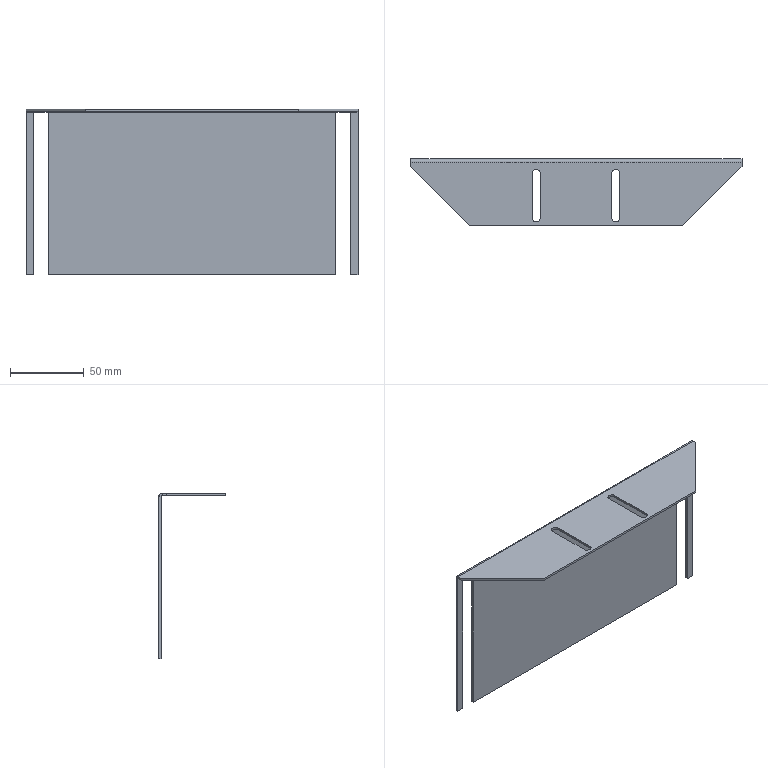Part | STEP file | A14-056 | 1 solid | 36 faces | box 225 x 45 x 112.237 mm | volume 46079 mm3 | plane 30 | cylinder 6 | commonest cylinder face diameters 5.5 x4 1.473 x1 4.473 x1